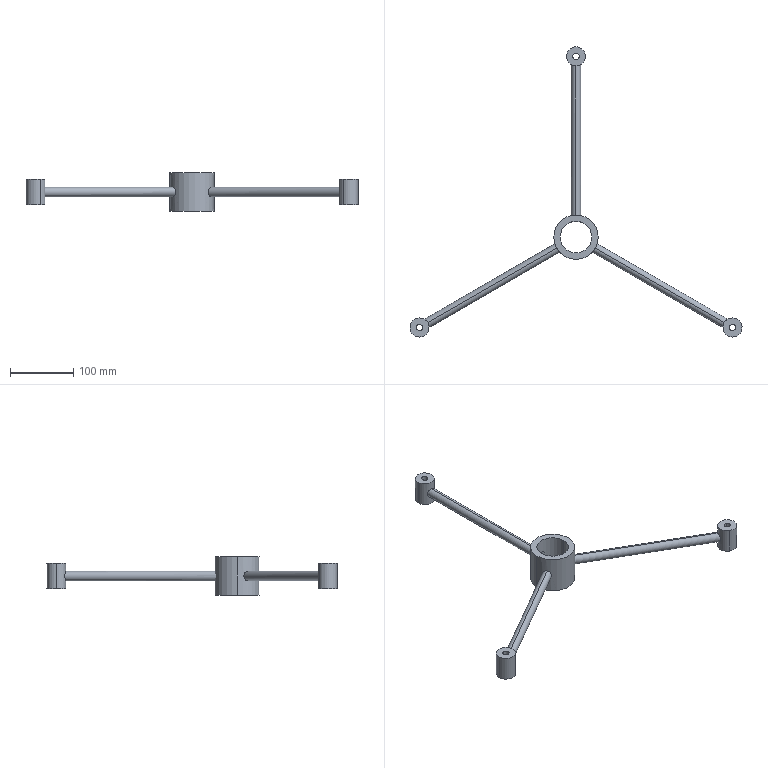Part | SolidWorks | features ICE 2, CirPattern 1, Extrusion 1 | 2 solids | 31 faces | box 523.634 x 457.5 x 60 mm | volume 315175 mm3 | cylinder 22 | plane 9 | commonest cylinder face diameters 10 x6 15 x6 30 x6 50 x2 70 x2
STEP:
#1=CARTESIAN_POINT('',(-5.,285.,20.));
#2=VERTEX_POINT('',#1);
#3=CARTESIAN_POINT('',(5.,285.,20.));
#4=VERTEX_POINT('',#3);
#5=CARTESIAN_POINT('',(0.,285.,20.));
#6=DIRECTION('',(0.,0.,1.));
#7=DIRECTION('',(1.,0.,0.));
#8=AXIS2_PLACEMENT_3D('',#5,#6,#7);
#9=CIRCLE('',#8,5.);
#10=EDGE_CURVE('',#2,#4,#9,.T.);
#11=ORIENTED_EDGE('',*,*,#10,.T.);
#12=CARTESIAN_POINT('',(5.,285.,-20.));
#13=VERTEX_POINT('',#12);
#14=CARTESIAN_POINT('',(5.,285.,20.));
#15=DIRECTION('',(0.,0.,-1.));
#16=VECTOR('',#15,1000.);
#17=LINE('',#14,#16);
#18=EDGE_CURVE('',#4,#13,#17,.T.);
#19=ORIENTED_EDGE('',*,*,#18,.T.);
#20=CARTESIAN_POINT('',(-5.,285.,-20.));
#21=VERTEX_POINT('',#20);
#22=CARTESIAN_POINT('',(0.,285.,-20.));
#23=DIRECTION('',(0.,0.,1.));
#24=DIRECTION('',(1.,0.,0.));
#25=AXIS2_PLACEMENT_3D('',#22,#23,#24);
#26=CIRCLE('',#25,5.);
#27=EDGE_CURVE('',#21,#13,#26,.T.);
#28=ORIENTED_EDGE('',*,*,#27,.F.);
#29=CARTESIAN_POINT('',(-5.,285.,20.));
#30=DIRECTION('',(0.,0.,-1.));
#31=VECTOR('',#30,1000.);
#32=LINE('',#29,#31);
#33=EDGE_CURVE('',#2,#21,#32,.T.);
#34=ORIENTED_EDGE('',*,*,#33,.F.);
#35=EDGE_LOOP('',(#11,#19,#28,#34));
#36=FACE_OUTER_BOUND('',#35,.T.);
#37=CARTESIAN_POINT('',(0.,285.,20.));
#38=DIRECTION('',(0.,0.,-1.));
#39=DIRECTION('',(-1.,0.,0.));
#40=AXIS2_PLACEMENT_3D('',#37,#38,#39);
#41=CYLINDRICAL_SURFACE('',#40,5.);
#42=ADVANCED_FACE('',(#36),#41,.F.);
#43=CARTESIAN_POINT('',(15.,285.,20.));
#44=VERTEX_POINT('',#43);
#45=CARTESIAN_POINT('',(-15.,285.,20.));
#46=VERTEX_POINT('',#45);
#47=CARTESIAN_POINT('',(0.,285.,20.));
#48=DIRECTION('',(0.,0.,1.));
#49=DIRECTION('',(1.,0.,0.));
#50=AXIS2_PLACEMENT_3D('',#47,#48,#49);
#51=CIRCLE('',#50,15.);
#52=EDGE_CURVE('',#44,#46,#51,.T.);
#53=ORIENTED_EDGE('',*,*,#52,.F.);
#54=CARTESIAN_POINT('',(15.,285.,-20.));
#55=VERTEX_POINT('',#54);
#56=CARTESIAN_POINT('',(15.,285.,20.));
#57=DIRECTION('',(0.,0.,-1.));
#58=VECTOR('',#57,1000.);
#59=LINE('',#56,#58);
#60=EDGE_CURVE('',#44,#55,#59,.T.);
#61=ORIENTED_EDGE('',*,*,#60,.T.);
#62=CARTESIAN_POINT('',(-15.,285.,-20.));
#63=VERTEX_POINT('',#62);
#64=CARTESIAN_POINT('',(0.,285.,-20.));
#65=DIRECTION('',(0.,0.,1.));
#66=DIRECTION('',(1.,0.,0.));
#67=AXIS2_PLACEMENT_3D('',#64,#65,#66);
#68=CIRCLE('',#67,15.);
#69=EDGE_CURVE('',#55,#63,#68,.T.);
#70=ORIENTED_EDGE('',*,*,#69,.T.);
#71=CARTESIAN_POINT('',(-15.,285.,20.));
#72=DIRECTION('',(0.,0.,-1.));
#73=VECTOR('',#72,1000.);
#74=LINE('',#71,#73);
#75=EDGE_CURVE('',#46,#63,#74,.T.);
#76=ORIENTED_EDGE('',*,*,#75,.F.);
#77=EDGE_LOOP('',(#53,#61,#70,#76));
#78=FACE_OUTER_BOUND('',#77,.T.);
#79=CARTESIAN_POINT('',(0.,285.,20.));
#80=DIRECTION('',(0.,0.,-1.));
#81=DIRECTION('',(-1.,0.,0.));
#82=AXIS2_PLACEMENT_3D('',#79,#80,#81);
#83=CYLINDRICAL_SURFACE('',#82,15.);
#84=ADVANCED_FACE('',(#78),#83,.T.);
#85=CARTESIAN_POINT('',(0.,270.,7.5));
#86=VERTEX_POINT('',#85);
#87=CARTESIAN_POINT('',(0.,270.,-7.5));
#88=VERTEX_POINT('',#87);
#89=CARTESIAN_POINT('',(0.,270.,7.5));
#90=CARTESIAN_POINT('',(0.4971,270.,7.5));
#91=CARTESIAN_POINT('',(1.003,270.026,7.449));
#92=CARTESIAN_POINT('',(1.975,270.123,7.252));
#93=CARTESIAN_POINT('',(2.446,270.193,7.107));
#94=CARTESIAN_POINT('',(3.36,270.374,6.724));
#95=CARTESIAN_POINT('',(3.789,270.48,6.491));
#96=CARTESIAN_POINT('',(4.592,270.714,5.949));
#97=CARTESIAN_POINT('',(4.97,270.843,5.637));
#98=CARTESIAN_POINT('',(5.651,271.1,4.955));
#99=CARTESIAN_POINT('',(5.956,271.23,4.584));
#100=CARTESIAN_POINT('',(6.361,271.415,3.981));
#101=CARTESIAN_POINT('',(6.488,271.475,3.771));
#102=CARTESIAN_POINT('',(6.719,271.588,3.341));
#103=CARTESIAN_POINT('',(6.824,271.642,3.122));
#104=CARTESIAN_POINT('',(7.105,271.788,2.449));
#105=CARTESIAN_POINT('',(7.251,271.868,1.982));
#106=CARTESIAN_POINT('',(7.4,271.952,1.248));
#107=CARTESIAN_POINT('',(7.437,271.974,0.999));
#108=CARTESIAN_POINT('',(7.487,272.002,0.5039));
#109=CARTESIAN_POINT('',(7.512,272.017,0.008359));
#110=CARTESIAN_POINT('',(7.488,272.003,-0.4882));
#111=CARTESIAN_POINT('',(7.439,271.975,-0.9852));
#112=CARTESIAN_POINT('',(7.402,271.953,-1.235));
#113=CARTESIAN_POINT('',(7.255,271.87,-1.967));
#114=CARTESIAN_POINT('',(7.11,271.79,-2.437));
#115=CARTESIAN_POINT('',(6.826,271.643,-3.117));
#116=CARTESIAN_POINT('',(6.719,271.589,-3.341));
#117=CARTESIAN_POINT('',(6.488,271.475,-3.77));
#118=CARTESIAN_POINT('',(6.363,271.416,-3.977));
#119=CARTESIAN_POINT('',(6.094,271.293,-4.379));
#120=CARTESIAN_POINT('',(5.95,271.23,-4.572));
#121=CARTESIAN_POINT('',(5.643,271.101,-4.946));
#122=CARTESIAN_POINT('',(5.479,271.035,-5.127));
#123=CARTESIAN_POINT('',(4.966,270.841,-5.641));
#124=CARTESIAN_POINT('',(4.595,270.715,-5.947));
#125=CARTESIAN_POINT('',(3.793,270.481,-6.488));
#126=CARTESIAN_POINT('',(3.356,270.373,-6.725));
#127=CARTESIAN_POINT('',(2.453,270.195,-7.105));
#128=CARTESIAN_POINT('',(1.984,270.124,-7.25));
#129=CARTESIAN_POINT('',(1.01,270.026,-7.448));
#130=CARTESIAN_POINT('',(0.5039,270.,-7.5));
#131=CARTESIAN_POINT('',(0.,270.,-7.5));
#132=B_SPLINE_CURVE_WITH_KNOTS('',3,(#89,#90,#91,#92,#93,#94,#95,#96,#97,#98,#99,#100,#101,#102,#103,#104,#105,#106,#107,#108,#109,#110,#111,#112,#113,#114,#115,#116,#117,#118,#119,#120,#121,#122,#123,#124,#125,#126,#127,#128,#129,#130,#131),.UNSPECIFIED.,.F.,.F.,(4,2,2,2,2,2,2,2,2,2,1,2,2,2,2,2,2,2,2,2,2,4),(0.02386,0.02535,0.02683,0.02832,0.02981,0.0313,0.03204,0.03279,0.03428,0.03502,0.03577,0.03651,0.03725,0.03874,0.03949,0.04023,0.04097,0.04172,0.04321,0.0447,0.04618,0.04767),.UNSPECIFIED.);
#133=EDGE_CURVE('',#86,#88,#132,.T.);
#134=ORIENTED_EDGE('',*,*,#133,.F.);
#135=CARTESIAN_POINT('',(0.,25.,7.5));
#136=VERTEX_POINT('',#135);
#137=CARTESIAN_POINT('',(0.,276.,7.5));
#138=DIRECTION('',(0.,-1.,0.));
#139=VECTOR('',#138,1000.);
#140=LINE('',#137,#139);
#141=EDGE_CURVE('',#86,#136,#140,.T.);
#142=ORIENTED_EDGE('',*,*,#141,.T.);
#143=CARTESIAN_POINT('',(0.,25.,-7.5));
#144=VERTEX_POINT('',#143);
#145=CARTESIAN_POINT('',(0.,25.,0.));
#146=DIRECTION('',(0.,1.,0.));
#147=DIRECTION('',(0.,0.,1.));
#148=AXIS2_PLACEMENT_3D('',#145,#146,#147);
#149=CIRCLE('',#148,7.5);
#150=EDGE_CURVE('',#136,#144,#149,.T.);
#151=ORIENTED_EDGE('',*,*,#150,.T.);
#152=CARTESIAN_POINT('',(0.,276.,-7.5));
#153=DIRECTION('',(0.,-1.,0.));
#154=VECTOR('',#153,1000.);
#155=LINE('',#152,#154);
#156=EDGE_CURVE('',#88,#144,#155,.T.);
#157=ORIENTED_EDGE('',*,*,#156,.F.);
#158=EDGE_LOOP('',(#134,#142,#151,#157));
#159=FACE_OUTER_BOUND('',#158,.T.);
#160=CARTESIAN_POINT('',(0.,276.,0.));
#161=DIRECTION('',(0.,-1.,0.));
#162=DIRECTION('',(0.,0.,-1.));
#163=AXIS2_PLACEMENT_3D('',#160,#161,#162);
#164=CYLINDRICAL_SURFACE('',#163,7.5);
#165=ADVANCED_FACE('',(#159),#164,.T.);
#166=ORIENTED_EDGE('',*,*,#141,.F.);
#167=CARTESIAN_POINT('',(0.,270.,-7.5));
#168=CARTESIAN_POINT('',(-0.5047,270.,-7.5));
#169=CARTESIAN_POINT('',(-0.9995,270.025,-7.45));
#170=CARTESIAN_POINT('',(-1.97,270.122,-7.253));
#171=CARTESIAN_POINT('',(-2.451,270.194,-7.105));
#172=CARTESIAN_POINT('',(-3.357,270.373,-6.725));
#173=CARTESIAN_POINT('',(-3.785,270.479,-6.493));
#174=CARTESIAN_POINT('',(-4.392,270.656,-6.084));
#175=CARTESIAN_POINT('',(-4.588,270.718,-5.938));
#176=CARTESIAN_POINT('',(-4.961,270.843,-5.63));
#177=CARTESIAN_POINT('',(-5.139,270.907,-5.468));
#178=CARTESIAN_POINT('',(-5.479,271.035,-5.127));
#179=CARTESIAN_POINT('',(-5.641,271.1,-4.949));
#180=CARTESIAN_POINT('',(-5.948,271.229,-4.575));
#181=CARTESIAN_POINT('',(-6.094,271.293,-4.379));
#182=CARTESIAN_POINT('',(-6.499,271.478,-3.774));
#183=CARTESIAN_POINT('',(-6.729,271.592,-3.348));
#184=CARTESIAN_POINT('',(-7.011,271.739,-2.675));
#185=CARTESIAN_POINT('',(-7.095,271.784,-2.444));
#186=CARTESIAN_POINT('',(-7.241,271.863,-1.97));
#187=CARTESIAN_POINT('',(-7.303,271.898,-1.727));
#188=CARTESIAN_POINT('',(-7.45,271.98,-0.9987));
#189=CARTESIAN_POINT('',(-7.5,272.009,-0.5064));
#190=CARTESIAN_POINT('',(-7.5,272.01,0.2423));
#191=CARTESIAN_POINT('',(-7.488,272.003,0.4954));
#192=CARTESIAN_POINT('',(-7.438,271.974,0.9943));
#193=CARTESIAN_POINT('',(-7.401,271.953,1.24));
#194=CARTESIAN_POINT('',(-7.303,271.898,1.726));
#195=CARTESIAN_POINT('',(-7.242,271.864,1.965));
#196=CARTESIAN_POINT('',(-7.097,271.785,2.437));
#197=CARTESIAN_POINT('',(-7.012,271.74,2.671));
#198=CARTESIAN_POINT('',(-6.727,271.591,3.352));
#199=CARTESIAN_POINT('',(-6.496,271.476,3.779));
#200=CARTESIAN_POINT('',(-6.09,271.291,4.384));
#201=CARTESIAN_POINT('',(-5.944,271.227,4.58));
#202=CARTESIAN_POINT('',(-5.636,271.098,4.954));
#203=CARTESIAN_POINT('',(-5.474,271.033,5.133));
#204=CARTESIAN_POINT('',(-4.964,270.84,5.643));
#205=CARTESIAN_POINT('',(-4.592,270.714,5.95));
#206=CARTESIAN_POINT('',(-3.779,270.478,6.497));
#207=CARTESIAN_POINT('',(-3.349,270.371,6.728));
#208=CARTESIAN_POINT('',(-2.674,270.238,7.011));
#209=CARTESIAN_POINT('',(-2.443,270.198,7.095));
#210=CARTESIAN_POINT('',(-1.971,270.128,7.241));
#211=CARTESIAN_POINT('',(-1.727,270.098,7.303));
#212=CARTESIAN_POINT('',(-0.9921,270.025,7.451));
#213=CARTESIAN_POINT('',(-0.498,270.,7.5));
#214=CARTESIAN_POINT('',(0.,270.,7.5));
#215=B_SPLINE_CURVE_WITH_KNOTS('',3,(#167,#168,#169,#170,#171,#172,#173,#174,#175,#176,#177,#178,#179,#180,#181,#182,#183,#184,#185,#186,#187,#188,#189,#190,#191,#192,#193,#194,#195,#196,#197,#198,#199,#200,#201,#202,#203,#204,#205,#206,#207,#208,#209,#210,#211,#212,#213,#214),.UNSPECIFIED.,.F.,.F.,(4,2,2,2,2,2,2,2,2,2,2,2,2,2,2,2,2,2,2,2,2,2,2,4),(0.,0.001491,0.002982,0.004473,0.005219,0.005964,0.00671,0.007455,0.008947,0.009692,0.01044,0.01193,0.01267,0.01342,0.01417,0.01491,0.0164,0.01715,0.01789,0.01938,0.02088,0.02162,0.02237,0.02386),.UNSPECIFIED.);
#216=EDGE_CURVE('',#88,#86,#215,.T.);
#217=ORIENTED_EDGE('',*,*,#216,.F.);
#218=ORIENTED_EDGE('',*,*,#156,.T.);
#219=CARTESIAN_POINT('',(0.,25.,0.));
#220=DIRECTION('',(0.,1.,0.));
#221=DIRECTION('',(0.,0.,1.));
#222=AXIS2_PLACEMENT_3D('',#219,#220,#221);
#223=CIRCLE('',#222,7.5);
#224=EDGE_CURVE('',#144,#136,#223,.T.);
#225=ORIENTED_EDGE('',*,*,#224,.T.);
#226=EDGE_LOOP('',(#166,#217,#218,#225));
#227=FACE_OUTER_BOUND('',#226,.T.);
#228=CARTESIAN_POINT('',(0.,276.,0.));
#229=DIRECTION('',(0.,-1.,0.));
#230=DIRECTION('',(0.,0.,-1.));
#231=AXIS2_PLACEMENT_3D('',#228,#229,#230);
#232=CYLINDRICAL_SURFACE('',#231,7.5);
#233=ADVANCED_FACE('',(#227),#232,.T.);
#234=ORIENTED_EDGE('',*,*,#224,.F.);
#235=ORIENTED_EDGE('',*,*,#150,.F.);
#236=EDGE_LOOP('',(#234,#235));
#237=FACE_OUTER_BOUND('',#236,.T.);
#238=CARTESIAN_POINT('',(0.,25.,0.));
#239=DIRECTION('',(0.,1.,0.));
#240=DIRECTION('',(0.,0.,1.));
#241=AXIS2_PLACEMENT_3D('',#238,#239,#240);
#242=PLANE('',#241);
#243=ADVANCED_FACE('',(#237),#242,.F.);
#244=ORIENTED_EDGE('',*,*,#60,.F.);
#245=CARTESIAN_POINT('',(0.,285.,20.));
#246=DIRECTION('',(0.,0.,1.));
#247=DIRECTION('',(1.,0.,0.));
#248=AXIS2_PLACEMENT_3D('',#245,#246,#247);
#249=CIRCLE('',#248,15.);
#250=EDGE_CURVE('',#46,#44,#249,.T.);
#251=ORIENTED_EDGE('',*,*,#250,.F.);
#252=ORIENTED_EDGE('',*,*,#75,.T.);
#253=CARTESIAN_POINT('',(0.,285.,-20.));
#254=DIRECTION('',(0.,0.,1.));
#255=DIRECTION('',(1.,0.,0.));
#256=AXIS2_PLACEMENT_3D('',#253,#254,#255);
#257=CIRCLE('',#256,15.);
#258=EDGE_CURVE('',#63,#55,#257,.T.);
#259=ORIENTED_EDGE('',*,*,#258,.T.);
#260=EDGE_LOOP('',(#244,#251,#252,#259));
#261=FACE_OUTER_BOUND('',#260,.T.);
#262=ORIENTED_EDGE('',*,*,#216,.T.);
#263=ORIENTED_EDGE('',*,*,#133,.T.);
#264=EDGE_LOOP('',(#262,#263));
#265=FACE_BOUND('',#264,.T.);
#266=CARTESIAN_POINT('',(0.,285.,20.));
#267=DIRECTION('',(0.,0.,-1.));
#268=DIRECTION('',(-1.,0.,0.));
#269=AXIS2_PLACEMENT_3D('',#266,#267,#268);
#270=CYLINDRICAL_SURFACE('',#269,15.);
#271=ADVANCED_FACE('',(#261,#265),#270,.T.);
#272=ORIENTED_EDGE('',*,*,#250,.T.);
#273=ORIENTED_EDGE('',*,*,#52,.T.);
#274=EDGE_LOOP('',(#272,#273));
#275=FACE_OUTER_BOUND('',#274,.T.);
#276=ORIENTED_EDGE('',*,*,#10,.F.);
#277=CARTESIAN_POINT('',(0.,285.,20.));
#278=DIRECTION('',(0.,0.,1.));
#279=DIRECTION('',(1.,0.,0.));
#280=AXIS2_PLACEMENT_3D('',#277,#278,#279);
#281=CIRCLE('',#280,5.);
#282=EDGE_CURVE('',#4,#2,#281,.T.);
#283=ORIENTED_EDGE('',*,*,#282,.F.);
#284=EDGE_LOOP('',(#276,#283));
#285=FACE_BOUND('',#284,.T.);
#286=CARTESIAN_POINT('',(0.,285.,20.));
#287=DIRECTION('',(0.,0.,1.));
#288=DIRECTION('',(1.,0.,0.));
#289=AXIS2_PLACEMENT_3D('',#286,#287,#288);
#290=PLANE('',#289);
#291=ADVANCED_FACE('',(#275,#285),#290,.T.);
#292=ORIENTED_EDGE('',*,*,#258,.F.);
#293=ORIENTED_EDGE('',*,*,#69,.F.);
#294=EDGE_LOOP('',(#292,#293));
#295=FACE_OUTER_BOUND('',#294,.T.);
#296=ORIENTED_EDGE('',*,*,#27,.T.);
#297=CARTESIAN_POINT('',(0.,285.,-20.));
#298=DIRECTION('',(0.,0.,1.));
#299=DIRECTION('',(1.,0.,0.));
#300=AXIS2_PLACEMENT_3D('',#297,#298,#299);
#301=CIRCLE('',#300,5.);
#302=EDGE_CURVE('',#13,#21,#301,.T.);
#303=ORIENTED_EDGE('',*,*,#302,.T.);
#304=EDGE_LOOP('',(#296,#303));
#305=FACE_BOUND('',#304,.T.);
#306=CARTESIAN_POINT('',(0.,285.,-20.));
#307=DIRECTION('',(0.,0.,1.));
#308=DIRECTION('',(1.,0.,0.));
#309=AXIS2_PLACEMENT_3D('',#306,#307,#308);
#310=PLANE('',#309);
#311=ADVANCED_FACE('',(#295,#305),#310,.F.);
#312=ORIENTED_EDGE('',*,*,#18,.F.);
#313=ORIENTED_EDGE('',*,*,#282,.T.);
#314=ORIENTED_EDGE('',*,*,#33,.T.);
#315=ORIENTED_EDGE('',*,*,#302,.F.);
#316=EDGE_LOOP('',(#312,#313,#314,#315));
#317=FACE_OUTER_BOUND('',#316,.T.);
#318=CARTESIAN_POINT('',(0.,285.,20.));
#319=DIRECTION('',(0.,0.,-1.));
#320=DIRECTION('',(-1.,0.,0.));
#321=AXIS2_PLACEMENT_3D('',#318,#319,#320);
#322=CYLINDRICAL_SURFACE('',#321,5.);
#323=ADVANCED_FACE('',(#317),#322,.F.);
#324=CLOSED_SHELL('',(#42,#84,#165,#233,#243,#271,#291,#311,#323));
#325=MANIFOLD_SOLID_BREP('',#324);
#326=CARTESIAN_POINT('',(-244.317,-146.83,20.));
#327=VERTEX_POINT('',#326);
#328=CARTESIAN_POINT('',(-249.317,-138.17,20.));
#329=VERTEX_POINT('',#328);
#330=CARTESIAN_POINT('',(-246.817,-142.5,20.));
#331=DIRECTION('',(0.,0.,1.));
#332=DIRECTION('',(-0.5,0.866,0.));
#333=AXIS2_PLACEMENT_3D('',#330,#331,#332);
#334=CIRCLE('',#333,5.);
#335=EDGE_CURVE('',#327,#329,#334,.T.);
#336=ORIENTED_EDGE('',*,*,#335,.T.);
#337=CARTESIAN_POINT('',(-249.317,-138.17,-20.));
#338=VERTEX_POINT('',#337);
#339=CARTESIAN_POINT('',(-249.317,-138.17,20.));
#340=DIRECTION('',(0.,0.,-1.));
#341=VECTOR('',#340,1000.);
#342=LINE('',#339,#341);
#343=EDGE_CURVE('',#329,#338,#342,.T.);
#344=ORIENTED_EDGE('',*,*,#343,.T.);
#345=CARTESIAN_POINT('',(-244.317,-146.83,-20.));
#346=VERTEX_POINT('',#345);
#347=CARTESIAN_POINT('',(-246.817,-142.5,-20.));
#348=DIRECTION('',(0.,0.,1.));
#349=DIRECTION('',(-0.5,0.866,0.));
#350=AXIS2_PLACEMENT_3D('',#347,#348,#349);
#351=CIRCLE('',#350,5.);
#352=EDGE_CURVE('',#346,#338,#351,.T.);
#353=ORIENTED_EDGE('',*,*,#352,.F.);
#354=CARTESIAN_POINT('',(-244.317,-146.83,20.));
#355=DIRECTION('',(0.,0.,-1.));
#356=VECTOR('',#355,1000.);
#357=LINE('',#354,#356);
#358=EDGE_CURVE('',#327,#346,#357,.T.);
#359=ORIENTED_EDGE('',*,*,#358,.F.);
#360=EDGE_LOOP('',(#336,#344,#353,#359));
#361=FACE_OUTER_BOUND('',#360,.T.);
#362=CARTESIAN_POINT('',(-246.817,-142.5,20.));
#363=DIRECTION('',(0.,0.,-1.));
#364=DIRECTION('',(0.5,-0.866,0.));
#365=AXIS2_PLACEMENT_3D('',#362,#363,#364);
#366=CYLINDRICAL_SURFACE('',#365,5.);
#367=ADVANCED_FACE('',(#361),#366,.F.);
#368=CARTESIAN_POINT('',(-254.317,-129.51,20.));
#369=VERTEX_POINT('',#368);
#370=CARTESIAN_POINT('',(-239.317,-155.49,20.));
#371=VERTEX_POINT('',#370);
#372=CARTESIAN_POINT('',(-246.817,-142.5,20.));
#373=DIRECTION('',(0.,0.,1.));
#374=DIRECTION('',(-0.5,0.866,0.));
#375=AXIS2_PLACEMENT_3D('',#372,#373,#374);
#376=CIRCLE('',#375,15.);
#377=EDGE_CURVE('',#369,#371,#376,.T.);
#378=ORIENTED_EDGE('',*,*,#377,.F.);
#379=CARTESIAN_POINT('',(-254.317,-129.51,-20.));
#380=VERTEX_POINT('',#379);
#381=CARTESIAN_POINT('',(-254.317,-129.51,20.));
#382=DIRECTION('',(0.,0.,-1.));
#383=VECTOR('',#382,1000.);
#384=LINE('',#381,#383);
#385=EDGE_CURVE('',#369,#380,#384,.T.);
#386=ORIENTED_EDGE('',*,*,#385,.T.);
#387=CARTESIAN_POINT('',(-239.317,-155.49,-20.));
#388=VERTEX_POINT('',#387);
#389=CARTESIAN_POINT('',(-246.817,-142.5,-20.));
#390=DIRECTION('',(0.,0.,1.));
#391=DIRECTION('',(-0.5,0.866,0.));
#392=AXIS2_PLACEMENT_3D('',#389,#390,#391);
#393=CIRCLE('',#392,15.);
#394=EDGE_CURVE('',#380,#388,#393,.T.);
#395=ORIENTED_EDGE('',*,*,#394,.T.);
#396=CARTESIAN_POINT('',(-239.317,-155.49,20.));
#397=DIRECTION('',(0.,0.,-1.));
#398=VECTOR('',#397,1000.);
#399=LINE('',#396,#398);
#400=EDGE_CURVE('',#371,#388,#399,.T.);
#401=ORIENTED_EDGE('',*,*,#400,.F.);
#402=EDGE_LOOP('',(#378,#386,#395,#401));
#403=FACE_OUTER_BOUND('',#402,.T.);
#404=CARTESIAN_POINT('',(-246.817,-142.5,20.));
#405=DIRECTION('',(0.,0.,-1.));
#406=DIRECTION('',(0.5,-0.866,0.));
#407=AXIS2_PLACEMENT_3D('',#404,#405,#406);
#408=CYLINDRICAL_SURFACE('',#407,15.);
#409=ADVANCED_FACE('',(#403),#408,.T.);
#410=CARTESIAN_POINT('',(-233.827,-135.,7.5));
#411=VERTEX_POINT('',#410);
#412=CARTESIAN_POINT('',(-233.827,-135.,-7.5));
#413=VERTEX_POINT('',#412);
#414=CARTESIAN_POINT('',(-233.827,-135.,7.5));
#415=CARTESIAN_POINT('',(-234.075,-134.569,7.5));
#416=CARTESIAN_POINT('',(-234.351,-134.144,7.449));
#417=CARTESIAN_POINT('',(-234.921,-133.351,7.252));
#418=CARTESIAN_POINT('',(-235.218,-132.978,7.107));
#419=CARTESIAN_POINT('',(-235.83,-132.277,6.724));
#420=CARTESIAN_POINT('',(-236.137,-131.959,6.491));
#421=CARTESIAN_POINT('',(-236.741,-131.38,5.949));
#422=CARTESIAN_POINT('',(-237.042,-131.117,5.637));
#423=CARTESIAN_POINT('',(-237.605,-130.656,4.955));
#424=CARTESIAN_POINT('',(-237.87,-130.457,4.584));
#425=CARTESIAN_POINT('',(-238.233,-130.199,3.981));
#426=CARTESIAN_POINT('',(-238.348,-130.119,3.771));
#427=CARTESIAN_POINT('',(-238.562,-129.975,3.341));
#428=CARTESIAN_POINT('',(-238.66,-129.911,3.122));
#429=CARTESIAN_POINT('',(-238.928,-129.74,2.449));
#430=CARTESIAN_POINT('',(-239.07,-129.655,1.982));
#431=CARTESIAN_POINT('',(-239.217,-129.568,1.248));
#432=CARTESIAN_POINT('',(-239.255,-129.546,0.999));
#433=CARTESIAN_POINT('',(-239.304,-129.517,0.5039));
#434=CARTESIAN_POINT('',(-239.33,-129.503,0.008359));
#435=CARTESIAN_POINT('',(-239.305,-129.516,-0.4882));
#436=CARTESIAN_POINT('',(-239.257,-129.545,-0.9852));
#437=CARTESIAN_POINT('',(-239.219,-129.567,-1.235));
#438=CARTESIAN_POINT('',(-239.074,-129.653,-1.967));
#439=CARTESIAN_POINT('',(-238.932,-129.738,-2.437));
#440=CARTESIAN_POINT('',(-238.662,-129.91,-3.117));
#441=CARTESIAN_POINT('',(-238.562,-129.975,-3.341));
#442=CARTESIAN_POINT('',(-238.349,-130.119,-3.77));
#443=CARTESIAN_POINT('',(-238.234,-130.197,-3.977));
#444=CARTESIAN_POINT('',(-237.994,-130.369,-4.379));
#445=CARTESIAN_POINT('',(-237.867,-130.462,-4.572));
#446=CARTESIAN_POINT('',(-237.602,-130.663,-4.946));
#447=CARTESIAN_POINT('',(-237.463,-130.773,-5.127));
#448=CARTESIAN_POINT('',(-237.039,-131.12,-5.641));
#449=CARTESIAN_POINT('',(-236.744,-131.378,-5.947));
#450=CARTESIAN_POINT('',(-236.14,-131.956,-6.488));
#451=CARTESIAN_POINT('',(-235.828,-132.28,-6.725));
#452=CARTESIAN_POINT('',(-235.222,-132.973,-7.105));
#453=CARTESIAN_POINT('',(-234.926,-133.344,-7.25));
#454=CARTESIAN_POINT('',(-234.355,-134.138,-7.448));
#455=CARTESIAN_POINT('',(-234.079,-134.564,-7.5));
#456=CARTESIAN_POINT('',(-233.827,-135.,-7.5));
#457=B_SPLINE_CURVE_WITH_KNOTS('',3,(#414,#415,#416,#417,#418,#419,#420,#421,#422,#423,#424,#425,#426,#427,#428,#429,#430,#431,#432,#433,#434,#435,#436,#437,#438,#439,#440,#441,#442,#443,#444,#445,#446,#447,#448,#449,#450,#451,#452,#453,#454,#455,#456),.UNSPECIFIED.,.F.,.F.,(4,2,2,2,2,2,2,2,2,2,1,2,2,2,2,2,2,2,2,2,2,4),(0.02386,0.02535,0.02683,0.02832,0.02981,0.0313,0.03204,0.03279,0.03428,0.03502,0.03577,0.03651,0.03725,0.03874,0.03949,0.04023,0.04097,0.04172,0.04321,0.0447,0.04618,0.04767),.UNSPECIFIED.);
#458=EDGE_CURVE('',#411,#413,#457,.T.);
#459=ORIENTED_EDGE('',*,*,#458,.F.);
#460=CARTESIAN_POINT('',(-30.311,-17.5,7.5));
#461=VERTEX_POINT('',#460);
#462=CARTESIAN_POINT('',(-239.023,-138.,7.5));
#463=DIRECTION('',(0.866,0.5,0.));
#464=VECTOR('',#463,1000.);
#465=LINE('',#462,#464);
#466=EDGE_CURVE('',#411,#461,#465,.T.);
#467=ORIENTED_EDGE('',*,*,#466,.T.);
#468=CARTESIAN_POINT('',(-30.311,-17.5,-7.5));
#469=VERTEX_POINT('',#468);
#470=CARTESIAN_POINT('',(-30.311,-17.5,7.5));
#471=CARTESIAN_POINT('',(-30.556,-17.076,7.5));
#472=CARTESIAN_POINT('',(-30.791,-16.648,7.452));
#473=CARTESIAN_POINT('',(-31.242,-15.785,7.259));
#474=CARTESIAN_POINT('',(-31.451,-15.363,7.115));
#475=CARTESIAN_POINT('',(-31.742,-14.748,6.834));
#476=CARTESIAN_POINT('',(-31.835,-14.546,6.73));
#477=CARTESIAN_POINT('',(-32.013,-14.149,6.498));
#478=CARTESIAN_POINT('',(-32.099,-13.953,6.37));
#479=CARTESIAN_POINT('',(-32.342,-13.386,5.961));
#480=CARTESIAN_POINT('',(-32.485,-13.034,5.652));
#481=CARTESIAN_POINT('',(-32.739,-12.382,4.961));
#482=CARTESIAN_POINT('',(-32.85,-12.081,4.576));
#483=CARTESIAN_POINT('',(-33.036,-11.562,3.765));
#484=CARTESIAN_POINT('',(-33.113,-11.34,3.335));
#485=CARTESIAN_POINT('',(-33.205,-11.065,2.652));
#486=CARTESIAN_POINT('',(-33.232,-10.984,2.418));
#487=CARTESIAN_POINT('',(-33.278,-10.845,1.948));
#488=CARTESIAN_POINT('',(-33.315,-10.729,1.473));
#489=CARTESIAN_POINT('',(-33.338,-10.658,0.9887));
#490=CARTESIAN_POINT('',(-33.353,-10.611,0.4994));
#491=CARTESIAN_POINT('',(-33.357,-10.598,0.2509));
#492=CARTESIAN_POINT('',(-33.357,-10.598,-0.4916));
#493=CARTESIAN_POINT('',(-33.342,-10.645,-0.9795));
#494=CARTESIAN_POINT('',(-33.282,-10.831,-1.941));
#495=CARTESIAN_POINT('',(-33.236,-10.972,-2.42));
#496=CARTESIAN_POINT('',(-33.114,-11.335,-3.325));
#497=CARTESIAN_POINT('',(-33.038,-11.557,-3.756));
#498=CARTESIAN_POINT('',(-32.898,-11.948,-4.368));
#499=CARTESIAN_POINT('',(-32.846,-12.089,-4.568));
#500=CARTESIAN_POINT('',(-32.736,-12.385,-4.947));
#501=CARTESIAN_POINT('',(-32.677,-12.54,-5.128));
#502=CARTESIAN_POINT('',(-32.487,-13.027,-5.645));
#503=CARTESIAN_POINT('',(-32.344,-13.38,-5.956));
#504=CARTESIAN_POINT('',(-32.019,-14.14,-6.506));
#505=CARTESIAN_POINT('',(-31.842,-14.535,-6.736));
#506=CARTESIAN_POINT('',(-31.552,-15.149,-7.018));
#507=CARTESIAN_POINT('',(-31.452,-15.357,-7.101));
#508=CARTESIAN_POINT('',(-31.241,-15.781,-7.245));
#509=CARTESIAN_POINT('',(-31.132,-15.996,-7.306));
#510=CARTESIAN_POINT('',(-30.795,-16.64,-7.451));
#511=CARTESIAN_POINT('',(-30.559,-17.07,-7.5));
#512=CARTESIAN_POINT('',(-30.311,-17.5,-7.5));
#513=B_SPLINE_CURVE_WITH_KNOTS('',3,(#470,#471,#472,#473,#474,#475,#476,#477,#478,#479,#480,#481,#482,#483,#484,#485,#486,#487,#488,#489,#490,#491,#492,#493,#494,#495,#496,#497,#498,#499,#500,#501,#502,#503,#504,#505,#506,#507,#508,#509,#510,#511,#512),.UNSPECIFIED.,.F.,.F.,(4,2,2,2,2,2,2,2,2,1,2,2,2,2,2,2,2,2,2,2,2,4),(0.02352,0.02499,0.02646,0.02719,0.02792,0.02939,0.03086,0.03233,0.03307,0.0338,0.03454,0.03527,0.03674,0.03821,0.03968,0.04041,0.04115,0.04262,0.04409,0.04482,0.04556,0.04703),.UNSPECIFIED.);
#514=EDGE_CURVE('',#461,#469,#513,.T.);
#515=ORIENTED_EDGE('',*,*,#514,.T.);
#516=CARTESIAN_POINT('',(-239.023,-138.,-7.5));
#517=DIRECTION('',(0.866,0.5,0.));
#518=VECTOR('',#517,1000.);
#519=LINE('',#516,#518);
#520=EDGE_CURVE('',#413,#469,#519,.T.);
#521=ORIENTED_EDGE('',*,*,#520,.F.);
#522=EDGE_LOOP('',(#459,#467,#515,#521));
#523=FACE_OUTER_BOUND('',#522,.T.);
#524=CARTESIAN_POINT('',(-239.023,-138.,0.));
#525=DIRECTION('',(0.866,0.5,0.));
#526=DIRECTION('',(0.,0.,-1.));
#527=AXIS2_PLACEMENT_3D('',#524,#525,#526);
#528=CYLINDRICAL_SURFACE('',#527,7.5);
#529=ADVANCED_FACE('',(#523),#528,.T.);
#530=CARTESIAN_POINT('',(249.317,-138.17,20.));
#531=VERTEX_POINT('',#530);
#532=CARTESIAN_POINT('',(244.317,-146.83,20.));
#533=VERTEX_POINT('',#532);
#534=CARTESIAN_POINT('',(246.817,-142.5,20.));
#535=DIRECTION('',(0.,0.,1.));
#536=DIRECTION('',(-0.5,-0.866,0.));
#537=AXIS2_PLACEMENT_3D('',#534,#535,#536);
#538=CIRCLE('',#537,5.);
#539=EDGE_CURVE('',#531,#533,#538,.T.);
#540=ORIENTED_EDGE('',*,*,#539,.T.);
#541=CARTESIAN_POINT('',(244.317,-146.83,-20.));
#542=VERTEX_POINT('',#541);
#543=CARTESIAN_POINT('',(244.317,-146.83,20.));
#544=DIRECTION('',(0.,0.,-1.));
#545=VECTOR('',#544,1000.);
#546=LINE('',#543,#545);
#547=EDGE_CURVE('',#533,#542,#546,.T.);
#548=ORIENTED_EDGE('',*,*,#547,.T.);
#549=CARTESIAN_POINT('',(249.317,-138.17,-20.));
#550=VERTEX_POINT('',#549);
#551=CARTESIAN_POINT('',(246.817,-142.5,-20.));
#552=DIRECTION('',(0.,0.,1.));
#553=DIRECTION('',(-0.5,-0.866,0.));
#554=AXIS2_PLACEMENT_3D('',#551,#552,#553);
#555=CIRCLE('',#554,5.);
#556=EDGE_CURVE('',#550,#542,#555,.T.);
#557=ORIENTED_EDGE('',*,*,#556,.F.);
#558=CARTESIAN_POINT('',(249.317,-138.17,20.));
#559=DIRECTION('',(0.,0.,-1.));
#560=VECTOR('',#559,1000.);
#561=LINE('',#558,#560);
#562=EDGE_CURVE('',#531,#550,#561,.T.);
#563=ORIENTED_EDGE('',*,*,#562,.F.);
#564=EDGE_LOOP('',(#540,#548,#557,#563));
#565=FACE_OUTER_BOUND('',#564,.T.);
#566=CARTESIAN_POINT('',(246.817,-142.5,20.));
#567=DIRECTION('',(0.,0.,-1.));
#568=DIRECTION('',(0.5,0.866,0.));
#569=AXIS2_PLACEMENT_3D('',#566,#567,#568);
#570=CYLINDRICAL_SURFACE('',#569,5.);
#571=ADVANCED_FACE('',(#565),#570,.F.);
#572=CARTESIAN_POINT('',(239.317,-155.49,20.));
#573=VERTEX_POINT('',#572);
#574=CARTESIAN_POINT('',(254.317,-129.51,20.));
#575=VERTEX_POINT('',#574);
#576=CARTESIAN_POINT('',(246.817,-142.5,20.));
#577=DIRECTION('',(0.,0.,1.));
#578=DIRECTION('',(-0.5,-0.866,0.));
#579=AXIS2_PLACEMENT_3D('',#576,#577,#578);
#580=CIRCLE('',#579,15.);
#581=EDGE_CURVE('',#573,#575,#580,.T.);
#582=ORIENTED_EDGE('',*,*,#581,.F.);
#583=CARTESIAN_POINT('',(239.317,-155.49,-20.));
#584=VERTEX_POINT('',#583);
#585=CARTESIAN_POINT('',(239.317,-155.49,20.));
#586=DIRECTION('',(0.,0.,-1.));
#587=VECTOR('',#586,1000.);
#588=LINE('',#585,#587);
#589=EDGE_CURVE('',#573,#584,#588,.T.);
#590=ORIENTED_EDGE('',*,*,#589,.T.);
#591=CARTESIAN_POINT('',(254.317,-129.51,-20.));
#592=VERTEX_POINT('',#591);
#593=CARTESIAN_POINT('',(246.817,-142.5,-20.));
#594=DIRECTION('',(0.,0.,1.));
#595=DIRECTION('',(-0.5,-0.866,0.));
#596=AXIS2_PLACEMENT_3D('',#593,#594,#595);
#597=CIRCLE('',#596,15.);
#598=EDGE_CURVE('',#584,#592,#597,.T.);
#599=ORIENTED_EDGE('',*,*,#598,.T.);
#600=CARTESIAN_POINT('',(254.317,-129.51,20.));
#601=DIRECTION('',(0.,0.,-1.));
#602=VECTOR('',#601,1000.);
#603=LINE('',#600,#602);
#604=EDGE_CURVE('',#575,#592,#603,.T.);
#605=ORIENTED_EDGE('',*,*,#604,.F.);
#606=EDGE_LOOP('',(#582,#590,#599,#605));
#607=FACE_OUTER_BOUND('',#606,.T.);
#608=CARTESIAN_POINT('',(246.817,-142.5,20.));
#609=DIRECTION('',(0.,0.,-1.));
#610=DIRECTION('',(0.5,0.866,0.));
#611=AXIS2_PLACEMENT_3D('',#608,#609,#610);
#612=CYLINDRICAL_SURFACE('',#611,15.);
#613=ADVANCED_FACE('',(#607),#612,.T.);
#614=CARTESIAN_POINT('',(233.827,-135.,7.5));
#615=VERTEX_POINT('',#614);
#616=CARTESIAN_POINT('',(233.827,-135.,-7.5));
#617=VERTEX_POINT('',#616);
#618=CARTESIAN_POINT('',(233.827,-135.,7.5));
#619=CARTESIAN_POINT('',(233.578,-135.431,7.5));
#620=CARTESIAN_POINT('',(233.348,-135.881,7.449));
#621=CARTESIAN_POINT('',(232.945,-136.772,7.252));
#622=CARTESIAN_POINT('',(232.771,-137.215,7.107));
#623=CARTESIAN_POINT('',(232.471,-138.097,6.724));
#624=CARTESIAN_POINT('',(232.348,-138.521,6.491));
#625=CARTESIAN_POINT('',(232.149,-139.334,5.949));
#626=CARTESIAN_POINT('',(232.072,-139.726,5.637));
#627=CARTESIAN_POINT('',(231.954,-140.444,4.955));
#628=CARTESIAN_POINT('',(231.914,-140.773,4.584));
#629=CARTESIAN_POINT('',(231.872,-141.216,3.981));
#630=CARTESIAN_POINT('',(231.86,-141.356,3.771));
#631=CARTESIAN_POINT('',(231.843,-141.613,3.341));
#632=CARTESIAN_POINT('',(231.837,-141.73,3.122));
#633=CARTESIAN_POINT('',(231.823,-142.048,2.449));
#634=CARTESIAN_POINT('',(231.82,-142.213,1.982));
#635=CARTESIAN_POINT('',(231.818,-142.384,1.248));
#636=CARTESIAN_POINT('',(231.817,-142.428,0.999));
#637=CARTESIAN_POINT('',(231.817,-142.485,0.5039));
#638=CARTESIAN_POINT('',(231.817,-142.514,0.008359));
#639=CARTESIAN_POINT('',(231.817,-142.486,-0.4882));
#640=CARTESIAN_POINT('',(231.817,-142.43,-0.9852));
#641=CARTESIAN_POINT('',(231.818,-142.387,-1.235));
#642=CARTESIAN_POINT('',(231.819,-142.218,-1.967));
#643=CARTESIAN_POINT('',(231.822,-142.053,-2.437));
#644=CARTESIAN_POINT('',(231.837,-141.733,-3.117));
#645=CARTESIAN_POINT('',(231.843,-141.613,-3.341));
#646=CARTESIAN_POINT('',(231.86,-141.357,-3.77));
#647=CARTESIAN_POINT('',(231.871,-141.218,-3.977));
#648=CARTESIAN_POINT('',(231.9,-140.924,-4.379));
#649=CARTESIAN_POINT('',(231.917,-140.768,-4.572));
#650=CARTESIAN_POINT('',(231.959,-140.437,-4.946));
#651=CARTESIAN_POINT('',(231.984,-140.263,-5.127));
#652=CARTESIAN_POINT('',(232.072,-139.722,-5.641));
#653=CARTESIAN_POINT('',(232.149,-139.337,-5.947));
#654=CARTESIAN_POINT('',(232.347,-138.525,-6.488));
#655=CARTESIAN_POINT('',(232.472,-138.093,-6.725));
#656=CARTESIAN_POINT('',(232.769,-137.221,-7.105));
#657=CARTESIAN_POINT('',(232.942,-136.78,-7.25));
#658=CARTESIAN_POINT('',(233.344,-135.888,-7.448));
#659=CARTESIAN_POINT('',(233.575,-135.436,-7.5));
#660=CARTESIAN_POINT('',(233.827,-135.,-7.5));
#661=B_SPLINE_CURVE_WITH_KNOTS('',3,(#618,#619,#620,#621,#622,#623,#624,#625,#626,#627,#628,#629,#630,#631,#632,#633,#634,#635,#636,#637,#638,#639,#640,#641,#642,#643,#644,#645,#646,#647,#648,#649,#650,#651,#652,#653,#654,#655,#656,#657,#658,#659,#660),.UNSPECIFIED.,.F.,.F.,(4,2,2,2,2,2,2,2,2,2,1,2,2,2,2,2,2,2,2,2,2,4),(0.02386,0.02535,0.02683,0.02832,0.02981,0.0313,0.03204,0.03279,0.03428,0.03502,0.03577,0.03651,0.03725,0.03874,0.03949,0.04023,0.04097,0.04172,0.04321,0.0447,0.04618,0.04767),.UNSPECIFIED.);
#662=EDGE_CURVE('',#615,#617,#661,.T.);
#663=ORIENTED_EDGE('',*,*,#662,.F.);
#664=CARTESIAN_POINT('',(30.311,-17.5,7.5));
#665=VERTEX_POINT('',#664);
#666=CARTESIAN_POINT('',(239.023,-138.,7.5));
#667=DIRECTION('',(-0.866,0.5,0.));
#668=VECTOR('',#667,1000.);
#669=LINE('',#666,#668);
#670=EDGE_CURVE('',#615,#665,#669,.T.);
#671=ORIENTED_EDGE('',*,*,#670,.T.);
#672=CARTESIAN_POINT('',(30.311,-17.5,-7.5));
#673=VERTEX_POINT('',#672);
#674=CARTESIAN_POINT('',(30.311,-17.5,7.5));
#675=CARTESIAN_POINT('',(30.066,-17.924,7.5));
#676=CARTESIAN_POINT('',(29.813,-18.342,7.452));
#677=CARTESIAN_POINT('',(29.291,-19.164,7.259));
#678=CARTESIAN_POINT('',(29.03,-19.556,7.115));
#679=CARTESIAN_POINT('',(28.643,-20.115,6.834));
#680=CARTESIAN_POINT('',(28.515,-20.297,6.73));
#681=CARTESIAN_POINT('',(28.26,-20.65,6.498));
#682=CARTESIAN_POINT('',(28.133,-20.823,6.37));
#683=CARTESIAN_POINT('',(27.764,-21.316,5.961));
#684=CARTESIAN_POINT('',(27.53,-21.616,5.652));
#685=CARTESIAN_POINT('',(27.092,-22.162,4.961));
#686=CARTESIAN_POINT('',(26.888,-22.408,4.576));
#687=CARTESIAN_POINT('',(26.531,-22.829,3.765));
#688=CARTESIAN_POINT('',(26.377,-23.007,3.335));
#689=CARTESIAN_POINT('',(26.185,-23.224,2.652));
#690=CARTESIAN_POINT('',(26.128,-23.288,2.418));
#691=CARTESIAN_POINT('',(26.031,-23.397,1.948));
#692=CARTESIAN_POINT('',(25.949,-23.487,1.473));
#693=CARTESIAN_POINT('',(25.899,-23.542,0.9887));
#694=CARTESIAN_POINT('',(25.866,-23.579,0.4994));
#695=CARTESIAN_POINT('',(25.857,-23.589,0.2509));
#696=CARTESIAN_POINT('',(25.857,-23.589,-0.4916));
#697=CARTESIAN_POINT('',(25.89,-23.552,-0.9795));
#698=CARTESIAN_POINT('',(26.021,-23.408,-1.941));
#699=CARTESIAN_POINT('',(26.12,-23.297,-2.42));
#700=CARTESIAN_POINT('',(26.374,-23.01,-3.325));
#701=CARTESIAN_POINT('',(26.528,-22.833,-3.756));
#702=CARTESIAN_POINT('',(26.796,-22.516,-4.368));
#703=CARTESIAN_POINT('',(26.893,-22.401,-4.568));
#704=CARTESIAN_POINT('',(27.093,-22.158,-4.947));
#705=CARTESIAN_POINT('',(27.198,-22.029,-5.128));
#706=CARTESIAN_POINT('',(27.525,-21.622,-5.645));
#707=CARTESIAN_POINT('',(27.76,-21.321,-5.956));
#708=CARTESIAN_POINT('',(28.255,-20.659,-6.506));
#709=CARTESIAN_POINT('',(28.509,-20.309,-6.736));
#710=CARTESIAN_POINT('',(28.896,-19.751,-7.018));
#711=CARTESIAN_POINT('',(29.026,-19.559,-7.101));
#712=CARTESIAN_POINT('',(29.287,-19.166,-7.245));
#713=CARTESIAN_POINT('',(29.419,-18.963,-7.306));
#714=CARTESIAN_POINT('',(29.808,-18.35,-7.451));
#715=CARTESIAN_POINT('',(30.062,-17.93,-7.5));
#716=CARTESIAN_POINT('',(30.311,-17.5,-7.5));
#717=B_SPLINE_CURVE_WITH_KNOTS('',3,(#674,#675,#676,#677,#678,#679,#680,#681,#682,#683,#684,#685,#686,#687,#688,#689,#690,#691,#692,#693,#694,#695,#696,#697,#698,#699,#700,#701,#702,#703,#704,#705,#706,#707,#708,#709,#710,#711,#712,#713,#714,#715,#716),.UNSPECIFIED.,.F.,.F.,(4,2,2,2,2,2,2,2,2,1,2,2,2,2,2,2,2,2,2,2,2,4),(0.02352,0.02499,0.02646,0.02719,0.02792,0.02939,0.03086,0.03233,0.03307,0.0338,0.03454,0.03527,0.03674,0.03821,0.03968,0.04041,0.04115,0.04262,0.04409,0.04482,0.04556,0.04703),.UNSPECIFIED.);
#718=EDGE_CURVE('',#665,#673,#717,.T.);
#719=ORIENTED_EDGE('',*,*,#718,.T.);
#720=CARTESIAN_POINT('',(239.023,-138.,-7.5));
#721=DIRECTION('',(-0.866,0.5,0.));
#722=VECTOR('',#721,1000.);
#723=LINE('',#720,#722);
#724=EDGE_CURVE('',#617,#673,#723,.T.);
#725=ORIENTED_EDGE('',*,*,#724,.F.);
#726=EDGE_LOOP('',(#663,#671,#719,#725));
#727=FACE_OUTER_BOUND('',#726,.T.);
#728=CARTESIAN_POINT('',(239.023,-138.,0.));
#729=DIRECTION('',(-0.866,0.5,0.));
#730=DIRECTION('',(0.,0.,-1.));
#731=AXIS2_PLACEMENT_3D('',#728,#729,#730);
#732=CYLINDRICAL_SURFACE('',#731,7.5);
#733=ADVANCED_FACE('',(#727),#732,.T.);
#734=CARTESIAN_POINT('',(-25.,0.,30.));
#735=VERTEX_POINT('',#734);
#736=CARTESIAN_POINT('',(25.,0.,30.));
#737=VERTEX_POINT('',#736);
#738=CARTESIAN_POINT('',(0.,0.,30.));
#739=DIRECTION('',(0.,0.,1.));
#740=DIRECTION('',(1.,0.,0.));
#741=AXIS2_PLACEMENT_3D('',#738,#739,#740);
#742=CIRCLE('',#741,25.);
#743=EDGE_CURVE('',#735,#737,#742,.T.);
#744=ORIENTED_EDGE('',*,*,#743,.T.);
#745=CARTESIAN_POINT('',(25.,0.,-30.));
#746=VERTEX_POINT('',#745);
#747=CARTESIAN_POINT('',(25.,0.,30.));
#748=DIRECTION('',(0.,0.,-1.));
#749=VECTOR('',#748,1000.);
#750=LINE('',#747,#749);
#751=EDGE_CURVE('',#737,#746,#750,.T.);
#752=ORIENTED_EDGE('',*,*,#751,.T.);
#753=CARTESIAN_POINT('',(-25.,0.,-30.));
#754=VERTEX_POINT('',#753);
#755=CARTESIAN_POINT('',(0.,0.,-30.));
#756=DIRECTION('',(0.,0.,1.));
#757=DIRECTION('',(1.,0.,0.));
#758=AXIS2_PLACEMENT_3D('',#755,#756,#757);
#759=CIRCLE('',#758,25.);
#760=EDGE_CURVE('',#754,#746,#759,.T.);
#761=ORIENTED_EDGE('',*,*,#760,.F.);
#762=CARTESIAN_POINT('',(-25.,0.,30.));
#763=DIRECTION('',(0.,0.,-1.));
#764=VECTOR('',#763,1000.);
#765=LINE('',#762,#764);
#766=EDGE_CURVE('',#735,#754,#765,.T.);
#767=ORIENTED_EDGE('',*,*,#766,.F.);
#768=EDGE_LOOP('',(#744,#752,#761,#767));
#769=FACE_OUTER_BOUND('',#768,.T.);
#770=CARTESIAN_POINT('',(0.,0.,30.));
#771=DIRECTION('',(0.,0.,-1.));
#772=DIRECTION('',(-1.,0.,0.));
#773=AXIS2_PLACEMENT_3D('',#770,#771,#772);
#774=CYLINDRICAL_SURFACE('',#773,25.);
#775=ADVANCED_FACE('',(#769),#774,.F.);
#776=CARTESIAN_POINT('',(35.,0.,30.));
#777=VERTEX_POINT('',#776);
#778=CARTESIAN_POINT('',(-35.,0.,30.));
#779=VERTEX_POINT('',#778);
#780=CARTESIAN_POINT('',(0.,0.,30.));
#781=DIRECTION('',(0.,0.,1.));
#782=DIRECTION('',(1.,0.,0.));
#783=AXIS2_PLACEMENT_3D('',#780,#781,#782);
#784=CIRCLE('',#783,35.);
#785=EDGE_CURVE('',#777,#779,#784,.T.);
#786=ORIENTED_EDGE('',*,*,#785,.F.);
#787=CARTESIAN_POINT('',(35.,0.,-30.));
#788=VERTEX_POINT('',#787);
#789=CARTESIAN_POINT('',(35.,0.,30.));
#790=DIRECTION('',(0.,0.,-1.));
#791=VECTOR('',#790,1000.);
#792=LINE('',#789,#791);
#793=EDGE_CURVE('',#777,#788,#792,.T.);
#794=ORIENTED_EDGE('',*,*,#793,.T.);
#795=CARTESIAN_POINT('',(-35.,0.,-30.));
#796=VERTEX_POINT('',#795);
#797=CARTESIAN_POINT('',(0.,0.,-30.));
#798=DIRECTION('',(0.,0.,1.));
#799=DIRECTION('',(1.,0.,0.));
#800=AXIS2_PLACEMENT_3D('',#797,#798,#799);
#801=CIRCLE('',#800,35.);
#802=EDGE_CURVE('',#788,#796,#801,.T.);
#803=ORIENTED_EDGE('',*,*,#802,.T.);
#804=CARTESIAN_POINT('',(-35.,0.,30.));
#805=DIRECTION('',(0.,0.,-1.));
#806=VECTOR('',#805,1000.);
#807=LINE('',#804,#806);
#808=EDGE_CURVE('',#779,#796,#807,.T.);
#809=ORIENTED_EDGE('',*,*,#808,.F.);
#810=EDGE_LOOP('',(#786,#794,#803,#809));
#811=FACE_OUTER_BOUND('',#810,.T.);
#812=CARTESIAN_POINT('',(0.,0.,30.));
#813=DIRECTION('',(0.,0.,-1.));
#814=DIRECTION('',(-1.,0.,0.));
#815=AXIS2_PLACEMENT_3D('',#812,#813,#814);
#816=CYLINDRICAL_SURFACE('',#815,35.);
#817=ADVANCED_FACE('',(#811),#816,.T.);
#818=ORIENTED_EDGE('',*,*,#793,.F.);
#819=CARTESIAN_POINT('',(0.,0.,30.));
#820=DIRECTION('',(0.,0.,1.));
#821=DIRECTION('',(1.,0.,0.));
#822=AXIS2_PLACEMENT_3D('',#819,#820,#821);
#823=CIRCLE('',#822,35.);
#824=EDGE_CURVE('',#779,#777,#823,.T.);
#825=ORIENTED_EDGE('',*,*,#824,.F.);
#826=ORIENTED_EDGE('',*,*,#808,.T.);
#827=CARTESIAN_POINT('',(0.,0.,-30.));
#828=DIRECTION('',(0.,0.,1.));
#829=DIRECTION('',(1.,0.,0.));
#830=AXIS2_PLACEMENT_3D('',#827,#828,#829);
#831=CIRCLE('',#830,35.);
#832=EDGE_CURVE('',#796,#788,#831,.T.);
#833=ORIENTED_EDGE('',*,*,#832,.T.);
#834=EDGE_LOOP('',(#818,#825,#826,#833));
#835=FACE_OUTER_BOUND('',#834,.T.);
#836=CARTESIAN_POINT('',(30.311,-17.5,-7.5));
#837=CARTESIAN_POINT('',(30.559,-17.07,-7.5));
#838=CARTESIAN_POINT('',(30.795,-16.641,-7.451));
#839=CARTESIAN_POINT('',(31.129,-16.002,-7.307));
#840=CARTESIAN_POINT('',(31.237,-15.79,-7.248));
#841=CARTESIAN_POINT('',(31.447,-15.366,-7.104));
#842=CARTESIAN_POINT('',(31.55,-15.155,-7.02));
#843=CARTESIAN_POINT('',(31.841,-14.537,-6.738));
#844=CARTESIAN_POINT('',(32.018,-14.142,-6.507));
#845=CARTESIAN_POINT('',(32.26,-13.577,-6.099));
#846=CARTESIAN_POINT('',(32.337,-13.392,-5.951));
#847=CARTESIAN_POINT('',(32.482,-13.036,-5.639));
#848=CARTESIAN_POINT('',(32.55,-12.866,-5.474));
#849=CARTESIAN_POINT('',(32.74,-12.379,-4.957));
#850=CARTESIAN_POINT('',(32.849,-12.084,-4.58));
#851=CARTESIAN_POINT('',(32.99,-11.691,-3.966));
#852=CARTESIAN_POINT('',(33.033,-11.569,-3.754));
#853=CARTESIAN_POINT('',(33.11,-11.346,-3.322));
#854=CARTESIAN_POINT('',(33.179,-11.145,-2.88));
#855=CARTESIAN_POINT('',(33.232,-10.984,-2.42));
#856=CARTESIAN_POINT('',(33.277,-10.845,-1.95));
#857=CARTESIAN_POINT('',(33.297,-10.786,-1.708));
#858=CARTESIAN_POINT('',(33.342,-10.645,-0.9814));
#859=CARTESIAN_POINT('',(33.357,-10.598,-0.4938));
#860=CARTESIAN_POINT('',(33.357,-10.598,0.4878));
#861=CARTESIAN_POINT('',(33.342,-10.646,0.9864));
#862=CARTESIAN_POINT('',(33.281,-10.833,1.95));
#863=CARTESIAN_POINT('',(33.236,-10.971,2.418));
#864=CARTESIAN_POINT('',(33.144,-11.245,3.1));
#865=CARTESIAN_POINT('',(33.11,-11.348,3.325));
#866=CARTESIAN_POINT('',(33.032,-11.571,3.758));
#867=CARTESIAN_POINT('',(32.99,-11.692,3.967));
#868=CARTESIAN_POINT('',(32.897,-11.951,4.373));
#869=CARTESIAN_POINT('',(32.846,-12.09,4.569));
#870=CARTESIAN_POINT('',(32.736,-12.385,4.947));
#871=CARTESIAN_POINT('',(32.676,-12.542,5.13));
#872=CARTESIAN_POINT('',(32.484,-13.034,5.652));
#873=CARTESIAN_POINT('',(32.341,-13.387,5.961));
#874=CARTESIAN_POINT('',(32.1,-13.95,6.369));
#875=CARTESIAN_POINT('',(32.016,-14.144,6.495));
#876=CARTESIAN_POINT('',(31.837,-14.542,6.728));
#877=CARTESIAN_POINT('',(31.742,-14.747,6.834));
#878=CARTESIAN_POINT('',(31.451,-15.363,7.116));
#879=CARTESIAN_POINT('',(31.243,-15.783,7.258));
#880=CARTESIAN_POINT('',(30.908,-16.425,7.403));
#881=CARTESIAN_POINT('',(30.791,-16.642,7.439));
#882=CARTESIAN_POINT('',(30.554,-17.074,7.488));
#883=CARTESIAN_POINT('',(30.433,-17.288,7.5));
#884=CARTESIAN_POINT('',(30.311,-17.5,7.5));
#885=B_SPLINE_CURVE_WITH_KNOTS('',3,(#836,#837,#838,#839,#840,#841,#842,#843,#844,#845,#846,#847,#848,#849,#850,#851,#852,#853,#854,#855,#856,#857,#858,#859,#860,#861,#862,#863,#864,#865,#866,#867,#868,#869,#870,#871,#872,#873,#874,#875,#876,#877,#878,#879,#880,#881,#882,#883,#884),.UNSPECIFIED.,.F.,.F.,(4,2,2,2,2,2,2,2,2,1,2,2,2,2,2,2,2,2,2,2,2,2,2,2,4),(0.,0.00147,0.002205,0.00294,0.004409,0.005144,0.005879,0.007349,0.008084,0.008819,0.009554,0.01029,0.01176,0.01323,0.0147,0.01543,0.01617,0.0169,0.01764,0.01911,0.01984,0.02058,0.02205,0.02278,0.02352),.UNSPECIFIED.);
#886=EDGE_CURVE('',#673,#665,#885,.T.);
#887=ORIENTED_EDGE('',*,*,#886,.F.);
#888=ORIENTED_EDGE('',*,*,#718,.F.);
#889=EDGE_LOOP('',(#887,#888));
#890=FACE_BOUND('',#889,.T.);
#891=CARTESIAN_POINT('',(-30.311,-17.5,-7.5));
#892=CARTESIAN_POINT('',(-30.062,-17.93,-7.5));
#893=CARTESIAN_POINT('',(-29.809,-18.348,-7.451));
#894=CARTESIAN_POINT('',(-29.423,-18.957,-7.307));
#895=CARTESIAN_POINT('',(-29.293,-19.157,-7.248));
#896=CARTESIAN_POINT('',(-29.031,-19.551,-7.104));
#897=CARTESIAN_POINT('',(-28.899,-19.745,-7.02));
#898=CARTESIAN_POINT('',(-28.51,-20.307,-6.738));
#899=CARTESIAN_POINT('',(-28.257,-20.657,-6.507));
#900=CARTESIAN_POINT('',(-27.888,-21.15,-6.099));
#901=CARTESIAN_POINT('',(-27.766,-21.309,-5.951));
#902=CARTESIAN_POINT('',(-27.531,-21.612,-5.639));
#903=CARTESIAN_POINT('',(-27.417,-21.756,-5.474));
#904=CARTESIAN_POINT('',(-27.09,-22.164,-4.957));
#905=CARTESIAN_POINT('',(-26.89,-22.406,-4.58));
#906=CARTESIAN_POINT('',(-26.62,-22.725,-3.966));
#907=CARTESIAN_POINT('',(-26.535,-22.823,-3.754));
#908=CARTESIAN_POINT('',(-26.381,-23.001,-3.322));
#909=CARTESIAN_POINT('',(-26.311,-23.081,-3.101));
#910=CARTESIAN_POINT('',(-26.185,-23.224,-2.65));
#911=CARTESIAN_POINT('',(-26.129,-23.287,-2.42));
#912=CARTESIAN_POINT('',(-26.031,-23.396,-1.95));
#913=CARTESIAN_POINT('',(-25.989,-23.443,-1.708));
#914=CARTESIAN_POINT('',(-25.89,-23.552,-0.9814));
#915=CARTESIAN_POINT('',(-25.857,-23.589,-0.4938));
#916=CARTESIAN_POINT('',(-25.857,-23.589,0.4878));
#917=CARTESIAN_POINT('',(-25.891,-23.552,0.9864));
#918=CARTESIAN_POINT('',(-26.023,-23.406,1.95));
#919=CARTESIAN_POINT('',(-26.12,-23.298,2.418));
#920=CARTESIAN_POINT('',(-26.311,-23.081,3.1));
#921=CARTESIAN_POINT('',(-26.382,-23.,3.325));
#922=CARTESIAN_POINT('',(-26.537,-22.821,3.758));
#923=CARTESIAN_POINT('',(-26.62,-22.724,3.967));
#924=CARTESIAN_POINT('',(-26.798,-22.514,4.373));
#925=CARTESIAN_POINT('',(-26.893,-22.401,4.569));
#926=CARTESIAN_POINT('',(-27.093,-22.158,4.947));
#927=CARTESIAN_POINT('',(-27.199,-22.028,5.13));
#928=CARTESIAN_POINT('',(-27.53,-21.615,5.652));
#929=CARTESIAN_POINT('',(-27.764,-21.315,5.961));
#930=CARTESIAN_POINT('',(-28.132,-20.825,6.369));
#931=CARTESIAN_POINT('',(-28.257,-20.654,6.495));
#932=CARTESIAN_POINT('',(-28.512,-20.3,6.728));
#933=CARTESIAN_POINT('',(-28.642,-20.116,6.834));
#934=CARTESIAN_POINT('',(-29.031,-19.556,7.116));
#935=CARTESIAN_POINT('',(-29.29,-19.166,7.258));
#936=CARTESIAN_POINT('',(-29.678,-18.554,7.403));
#937=CARTESIAN_POINT('',(-29.808,-18.345,7.439));
#938=CARTESIAN_POINT('',(-30.063,-17.924,7.488));
#939=CARTESIAN_POINT('',(-30.188,-17.712,7.5));
#940=CARTESIAN_POINT('',(-30.311,-17.5,7.5));
#941=B_SPLINE_CURVE_WITH_KNOTS('',3,(#891,#892,#893,#894,#895,#896,#897,#898,#899,#900,#901,#902,#903,#904,#905,#906,#907,#908,#909,#910,#911,#912,#913,#914,#915,#916,#917,#918,#919,#920,#921,#922,#923,#924,#925,#926,#927,#928,#929,#930,#931,#932,#933,#934,#935,#936,#937,#938,#939,#940),.UNSPECIFIED.,.F.,.F.,(4,2,2,2,2,2,2,2,2,2,2,2,2,2,2,2,2,2,2,2,2,2,2,2,4),(0.,0.00147,0.002205,0.00294,0.004409,0.005144,0.005879,0.007349,0.008084,0.008819,0.009554,0.01029,0.01176,0.01323,0.0147,0.01543,0.01617,0.0169,0.01764,0.01911,0.01984,0.02058,0.02205,0.02278,0.02352),.UNSPECIFIED.);
#942=EDGE_CURVE('',#469,#461,#941,.T.);
#943=ORIENTED_EDGE('',*,*,#942,.F.);
#944=ORIENTED_EDGE('',*,*,#514,.F.);
#945=EDGE_LOOP('',(#943,#944));
#946=FACE_BOUND('',#945,.T.);
#947=CARTESIAN_POINT('',(0.,0.,30.));
#948=DIRECTION('',(0.,0.,-1.));
#949=DIRECTION('',(-1.,0.,0.));
#950=AXIS2_PLACEMENT_3D('',#947,#948,#949);
#951=CYLINDRICAL_SURFACE('',#950,35.);
#952=ADVANCED_FACE('',(#835,#890,#946),#951,.T.);
#953=ORIENTED_EDGE('',*,*,#824,.T.);
#954=ORIENTED_EDGE('',*,*,#785,.T.);
#955=EDGE_LOOP('',(#953,#954));
#956=FACE_OUTER_BOUND('',#955,.T.);
#957=ORIENTED_EDGE('',*,*,#743,.F.);
#958=CARTESIAN_POINT('',(0.,0.,30.));
#959=DIRECTION('',(0.,0.,1.));
#960=DIRECTION('',(1.,0.,0.));
#961=AXIS2_PLACEMENT_3D('',#958,#959,#960);
#962=CIRCLE('',#961,25.);
#963=EDGE_CURVE('',#737,#735,#962,.T.);
#964=ORIENTED_EDGE('',*,*,#963,.F.);
#965=EDGE_LOOP('',(#957,#964));
#966=FACE_BOUND('',#965,.T.);
#967=CARTESIAN_POINT('',(0.,0.,30.));
#968=DIRECTION('',(0.,0.,1.));
#969=DIRECTION('',(1.,0.,0.));
#970=AXIS2_PLACEMENT_3D('',#967,#968,#969);
#971=PLANE('',#970);
#972=ADVANCED_FACE('',(#956,#966),#971,.T.);
#973=ORIENTED_EDGE('',*,*,#832,.F.);
#974=ORIENTED_EDGE('',*,*,#802,.F.);
#975=EDGE_LOOP('',(#973,#974));
#976=FACE_OUTER_BOUND('',#975,.T.);
#977=ORIENTED_EDGE('',*,*,#760,.T.);
#978=CARTESIAN_POINT('',(0.,0.,-30.));
#979=DIRECTION('',(0.,0.,1.));
#980=DIRECTION('',(1.,0.,0.));
#981=AXIS2_PLACEMENT_3D('',#978,#979,#980);
#982=CIRCLE('',#981,25.);
#983=EDGE_CURVE('',#746,#754,#982,.T.);
#984=ORIENTED_EDGE('',*,*,#983,.T.);
#985=EDGE_LOOP('',(#977,#984));
#986=FACE_BOUND('',#985,.T.);
#987=CARTESIAN_POINT('',(0.,0.,-30.));
#988=DIRECTION('',(0.,0.,1.));
#989=DIRECTION('',(1.,0.,0.));
#990=AXIS2_PLACEMENT_3D('',#987,#988,#989);
#991=PLANE('',#990);
#992=ADVANCED_FACE('',(#976,#986),#991,.F.);
#993=ORIENTED_EDGE('',*,*,#751,.F.);
#994=ORIENTED_EDGE('',*,*,#963,.T.);
#995=ORIENTED_EDGE('',*,*,#766,.T.);
#996=ORIENTED_EDGE('',*,*,#983,.F.);
#997=EDGE_LOOP('',(#993,#994,#995,#996));
#998=FACE_OUTER_BOUND('',#997,.T.);
#999=CARTESIAN_POINT('',(0.,0.,30.));
#1000=DIRECTION('',(0.,0.,-1.));
#1001=DIRECTION('',(-1.,0.,0.));
#1002=AXIS2_PLACEMENT_3D('',#999,#1000,#1001);
#1003=CYLINDRICAL_SURFACE('',#1002,25.);
#1004=ADVANCED_FACE('',(#998),#1003,.F.);
#1005=ORIENTED_EDGE('',*,*,#670,.F.);
#1006=CARTESIAN_POINT('',(233.827,-135.,-7.5));
#1007=CARTESIAN_POINT('',(234.079,-134.563,-7.5));
#1008=CARTESIAN_POINT('',(234.349,-134.147,-7.45));
#1009=CARTESIAN_POINT('',(234.918,-133.355,-7.253));
#1010=CARTESIAN_POINT('',(235.221,-132.974,-7.105));
#1011=CARTESIAN_POINT('',(235.829,-132.279,-6.725));
#1012=CARTESIAN_POINT('',(236.134,-131.962,-6.493));
#1013=CARTESIAN_POINT('',(236.591,-131.524,-6.084));
#1014=CARTESIAN_POINT('',(236.742,-131.385,-5.938));
#1015=CARTESIAN_POINT('',(237.038,-131.125,-5.63));
#1016=CARTESIAN_POINT('',(237.182,-131.002,-5.468));
#1017=CARTESIAN_POINT('',(237.463,-130.773,-5.127));
#1018=CARTESIAN_POINT('',(237.6,-130.665,-4.949));
#1019=CARTESIAN_POINT('',(237.865,-130.463,-4.575));
#1020=CARTESIAN_POINT('',(237.993,-130.369,-4.379));
#1021=CARTESIAN_POINT('',(238.357,-130.11,-3.774));
#1022=CARTESIAN_POINT('',(238.57,-129.969,-3.348));
#1023=CARTESIAN_POINT('',(238.838,-129.798,-2.675));
#1024=CARTESIAN_POINT('',(238.919,-129.747,-2.444));
#1025=CARTESIAN_POINT('',(239.061,-129.661,-1.97));
#1026=CARTESIAN_POINT('',(239.121,-129.625,-1.727));
#1027=CARTESIAN_POINT('',(239.267,-129.538,-0.9987));
#1028=CARTESIAN_POINT('',(239.317,-129.51,-0.5064));
#1029=CARTESIAN_POINT('',(239.317,-129.509,0.2423));
#1030=CARTESIAN_POINT('',(239.305,-129.517,0.4954));
#1031=CARTESIAN_POINT('',(239.255,-129.545,0.9943));
#1032=CARTESIAN_POINT('',(239.218,-129.567,1.24));
#1033=CARTESIAN_POINT('',(239.122,-129.624,1.726));
#1034=CARTESIAN_POINT('',(239.062,-129.66,1.965));
#1035=CARTESIAN_POINT('',(238.921,-129.746,2.437));
#1036=CARTESIAN_POINT('',(238.84,-129.797,2.671));
#1037=CARTESIAN_POINT('',(238.569,-129.97,3.352));
#1038=CARTESIAN_POINT('',(238.354,-130.112,3.779));
#1039=CARTESIAN_POINT('',(237.99,-130.371,4.384));
#1040=CARTESIAN_POINT('',(237.862,-130.466,4.58));
#1041=CARTESIAN_POINT('',(237.596,-130.668,4.954));
#1042=CARTESIAN_POINT('',(237.459,-130.776,5.133));
#1043=CARTESIAN_POINT('',(237.036,-131.122,5.643));
#1044=CARTESIAN_POINT('',(236.741,-131.38,5.95));
#1045=CARTESIAN_POINT('',(236.13,-131.966,6.497));
#1046=CARTESIAN_POINT('',(235.823,-132.285,6.728));
#1047=CARTESIAN_POINT('',(235.37,-132.804,7.011));
#1048=CARTESIAN_POINT('',(235.22,-132.983,7.095));
#1049=CARTESIAN_POINT('',(234.923,-133.357,7.241));
#1050=CARTESIAN_POINT('',(234.775,-133.553,7.303));
#1051=CARTESIAN_POINT('',(234.344,-134.153,7.451));
#1052=CARTESIAN_POINT('',(234.076,-134.569,7.5));
#1053=CARTESIAN_POINT('',(233.827,-135.,7.5));
#1054=B_SPLINE_CURVE_WITH_KNOTS('',3,(#1006,#1007,#1008,#1009,#1010,#1011,#1012,#1013,#1014,#1015,#1016,#1017,#1018,#1019,#1020,#1021,#1022,#1023,#1024,#1025,#1026,#1027,#1028,#1029,#1030,#1031,#1032,#1033,#1034,#1035,#1036,#1037,#1038,#1039,#1040,#1041,#1042,#1043,#1044,#1045,#1046,#1047,#1048,#1049,#1050,#1051,#1052,#1053),.UNSPECIFIED.,.F.,.F.,(4,2,2,2,2,2,2,2,2,2,2,2,2,2,2,2,2,2,2,2,2,2,2,4),(0.,0.001491,0.002982,0.004473,0.005219,0.005964,0.00671,0.007455,0.008947,0.009692,0.01044,0.01193,0.01267,0.01342,0.01417,0.01491,0.0164,0.01715,0.01789,0.01938,0.02088,0.02162,0.02237,0.02386),.UNSPECIFIED.);
#1055=EDGE_CURVE('',#617,#615,#1054,.T.);
#1056=ORIENTED_EDGE('',*,*,#1055,.F.);
#1057=ORIENTED_EDGE('',*,*,#724,.T.);
#1058=ORIENTED_EDGE('',*,*,#886,.T.);
#1059=EDGE_LOOP('',(#1005,#1056,#1057,#1058));
#1060=FACE_OUTER_BOUND('',#1059,.T.);
#1061=CARTESIAN_POINT('',(239.023,-138.,0.));
#1062=DIRECTION('',(-0.866,0.5,0.));
#1063=DIRECTION('',(0.,0.,-1.));
#1064=AXIS2_PLACEMENT_3D('',#1061,#1062,#1063);
#1065=CYLINDRICAL_SURFACE('',#1064,7.5);
#1066=ADVANCED_FACE('',(#1060),#1065,.T.);
#1067=ORIENTED_EDGE('',*,*,#547,.F.);
#1068=CARTESIAN_POINT('',(246.817,-142.5,20.));
#1069=DIRECTION('',(0.,0.,1.));
#1070=DIRECTION('',(-0.5,-0.866,0.));
#1071=AXIS2_PLACEMENT_3D('',#1068,#1069,#1070);
#1072=CIRCLE('',#1071,5.);
#1073=EDGE_CURVE('',#533,#531,#1072,.T.);
#1074=ORIENTED_EDGE('',*,*,#1073,.T.);
#1075=ORIENTED_EDGE('',*,*,#562,.T.);
#1076=CARTESIAN_POINT('',(246.817,-142.5,-20.));
#1077=DIRECTION('',(0.,0.,1.));
#1078=DIRECTION('',(-0.5,-0.866,0.));
#1079=AXIS2_PLACEMENT_3D('',#1076,#1077,#1078);
#1080=CIRCLE('',#1079,5.);
#1081=EDGE_CURVE('',#542,#550,#1080,.T.);
#1082=ORIENTED_EDGE('',*,*,#1081,.F.);
#1083=EDGE_LOOP('',(#1067,#1074,#1075,#1082));
#1084=FACE_OUTER_BOUND('',#1083,.T.);
#1085=CARTESIAN_POINT('',(246.817,-142.5,20.));
#1086=DIRECTION('',(0.,0.,-1.));
#1087=DIRECTION('',(0.5,0.866,0.));
#1088=AXIS2_PLACEMENT_3D('',#1085,#1086,#1087);
#1089=CYLINDRICAL_SURFACE('',#1088,5.);
#1090=ADVANCED_FACE('',(#1084),#1089,.F.);
#1091=CARTESIAN_POINT('',(246.817,-142.5,-20.));
#1092=DIRECTION('',(0.,0.,1.));
#1093=DIRECTION('',(-0.5,-0.866,0.));
#1094=AXIS2_PLACEMENT_3D('',#1091,#1092,#1093);
#1095=CIRCLE('',#1094,15.);
#1096=EDGE_CURVE('',#592,#584,#1095,.T.);
#1097=ORIENTED_EDGE('',*,*,#1096,.F.);
#1098=ORIENTED_EDGE('',*,*,#598,.F.);
#1099=EDGE_LOOP('',(#1097,#1098));
#1100=FACE_OUTER_BOUND('',#1099,.T.);
#1101=ORIENTED_EDGE('',*,*,#556,.T.);
#1102=ORIENTED_EDGE('',*,*,#1081,.T.);
#1103=EDGE_LOOP('',(#1101,#1102));
#1104=FACE_BOUND('',#1103,.T.);
#1105=CARTESIAN_POINT('',(246.817,-142.5,-20.));
#1106=DIRECTION('',(0.,0.,1.));
#1107=DIRECTION('',(-0.5,-0.866,0.));
#1108=AXIS2_PLACEMENT_3D('',#1105,#1106,#1107);
#1109=PLANE('',#1108);
#1110=ADVANCED_FACE('',(#1100,#1104),#1109,.F.);
#1111=CARTESIAN_POINT('',(246.817,-142.5,20.));
#1112=DIRECTION('',(0.,0.,1.));
#1113=DIRECTION('',(-0.5,-0.866,0.));
#1114=AXIS2_PLACEMENT_3D('',#1111,#1112,#1113);
#1115=CIRCLE('',#1114,15.);
#1116=EDGE_CURVE('',#575,#573,#1115,.T.);
#1117=ORIENTED_EDGE('',*,*,#1116,.T.);
#1118=ORIENTED_EDGE('',*,*,#581,.T.);
#1119=EDGE_LOOP('',(#1117,#1118));
#1120=FACE_OUTER_BOUND('',#1119,.T.);
#1121=ORIENTED_EDGE('',*,*,#539,.F.);
#1122=ORIENTED_EDGE('',*,*,#1073,.F.);
#1123=EDGE_LOOP('',(#1121,#1122));
#1124=FACE_BOUND('',#1123,.T.);
#1125=CARTESIAN_POINT('',(246.817,-142.5,20.));
#1126=DIRECTION('',(0.,0.,1.));
#1127=DIRECTION('',(-0.5,-0.866,0.));
#1128=AXIS2_PLACEMENT_3D('',#1125,#1126,#1127);
#1129=PLANE('',#1128);
#1130=ADVANCED_FACE('',(#1120,#1124),#1129,.T.);
#1131=ORIENTED_EDGE('',*,*,#589,.F.);
#1132=ORIENTED_EDGE('',*,*,#1116,.F.);
#1133=ORIENTED_EDGE('',*,*,#604,.T.);
#1134=ORIENTED_EDGE('',*,*,#1096,.T.);
#1135=EDGE_LOOP('',(#1131,#1132,#1133,#1134));
#1136=FACE_OUTER_BOUND('',#1135,.T.);
#1137=ORIENTED_EDGE('',*,*,#1055,.T.);
#1138=ORIENTED_EDGE('',*,*,#662,.T.);
#1139=EDGE_LOOP('',(#1137,#1138));
#1140=FACE_BOUND('',#1139,.T.);
#1141=CARTESIAN_POINT('',(246.817,-142.5,20.));
#1142=DIRECTION('',(0.,0.,-1.));
#1143=DIRECTION('',(0.5,0.866,0.));
#1144=AXIS2_PLACEMENT_3D('',#1141,#1142,#1143);
#1145=CYLINDRICAL_SURFACE('',#1144,15.);
#1146=ADVANCED_FACE('',(#1136,#1140),#1145,.T.);
#1147=ORIENTED_EDGE('',*,*,#466,.F.);
#1148=CARTESIAN_POINT('',(-233.827,-135.,-7.5));
#1149=CARTESIAN_POINT('',(-233.574,-135.437,-7.5));
#1150=CARTESIAN_POINT('',(-233.349,-135.878,-7.45));
#1151=CARTESIAN_POINT('',(-232.947,-136.767,-7.253));
#1152=CARTESIAN_POINT('',(-232.77,-137.22,-7.105));
#1153=CARTESIAN_POINT('',(-232.472,-138.094,-6.725));
#1154=CARTESIAN_POINT('',(-232.349,-138.518,-6.493));
#1155=CARTESIAN_POINT('',(-232.199,-139.132,-6.084));
#1156=CARTESIAN_POINT('',(-232.154,-139.332,-5.938));
#1157=CARTESIAN_POINT('',(-232.076,-139.718,-5.63));
#1158=CARTESIAN_POINT('',(-232.042,-139.904,-5.468));
#1159=CARTESIAN_POINT('',(-231.984,-140.263,-5.127));
#1160=CARTESIAN_POINT('',(-231.959,-140.435,-4.949));
#1161=CARTESIAN_POINT('',(-231.917,-140.765,-4.575));
#1162=CARTESIAN_POINT('',(-231.9,-140.923,-4.379));
#1163=CARTESIAN_POINT('',(-231.857,-141.368,-3.774));
#1164=CARTESIAN_POINT('',(-231.841,-141.623,-3.348));
#1165=CARTESIAN_POINT('',(-231.827,-141.941,-2.675));
#1166=CARTESIAN_POINT('',(-231.824,-142.036,-2.444));
#1167=CARTESIAN_POINT('',(-231.82,-142.202,-1.97));
#1168=CARTESIAN_POINT('',(-231.819,-142.273,-1.727));
#1169=CARTESIAN_POINT('',(-231.817,-142.442,-0.9987));
#1170=CARTESIAN_POINT('',(-231.817,-142.499,-0.5064));
#1171=CARTESIAN_POINT('',(-231.817,-142.5,0.2423));
#1172=CARTESIAN_POINT('',(-231.817,-142.486,0.4954));
#1173=CARTESIAN_POINT('',(-231.817,-142.429,0.9943));
#1174=CARTESIAN_POINT('',(-231.818,-142.386,1.24));
#1175=CARTESIAN_POINT('',(-231.819,-142.273,1.726));
#1176=CARTESIAN_POINT('',(-231.82,-142.204,1.965));
#1177=CARTESIAN_POINT('',(-231.824,-142.039,2.437));
#1178=CARTESIAN_POINT('',(-231.827,-141.943,2.671));
#1179=CARTESIAN_POINT('',(-231.841,-141.621,3.352));
#1180=CARTESIAN_POINT('',(-231.857,-141.364,3.779));
#1181=CARTESIAN_POINT('',(-231.9,-140.92,4.384));
#1182=CARTESIAN_POINT('',(-231.917,-140.762,4.58));
#1183=CARTESIAN_POINT('',(-231.96,-140.43,4.954));
#1184=CARTESIAN_POINT('',(-231.985,-140.257,5.133));
#1185=CARTESIAN_POINT('',(-232.073,-139.719,5.643));
#1186=CARTESIAN_POINT('',(-232.149,-139.334,5.95));
#1187=CARTESIAN_POINT('',(-232.351,-138.512,6.497));
#1188=CARTESIAN_POINT('',(-232.474,-138.086,6.728));
#1189=CARTESIAN_POINT('',(-232.696,-137.435,7.011));
#1190=CARTESIAN_POINT('',(-232.777,-137.215,7.095));
#1191=CARTESIAN_POINT('',(-232.952,-136.771,7.241));
#1192=CARTESIAN_POINT('',(-233.048,-136.545,7.303));
#1193=CARTESIAN_POINT('',(-233.352,-135.872,7.451));
#1194=CARTESIAN_POINT('',(-233.578,-135.431,7.5));
#1195=CARTESIAN_POINT('',(-233.827,-135.,7.5));
#1196=B_SPLINE_CURVE_WITH_KNOTS('',3,(#1148,#1149,#1150,#1151,#1152,#1153,#1154,#1155,#1156,#1157,#1158,#1159,#1160,#1161,#1162,#1163,#1164,#1165,#1166,#1167,#1168,#1169,#1170,#1171,#1172,#1173,#1174,#1175,#1176,#1177,#1178,#1179,#1180,#1181,#1182,#1183,#1184,#1185,#1186,#1187,#1188,#1189,#1190,#1191,#1192,#1193,#1194,#1195),.UNSPECIFIED.,.F.,.F.,(4,2,2,2,2,2,2,2,2,2,2,2,2,2,2,2,2,2,2,2,2,2,2,4),(0.,0.001491,0.002982,0.004473,0.005219,0.005964,0.00671,0.007455,0.008947,0.009692,0.01044,0.01193,0.01267,0.01342,0.01417,0.01491,0.0164,0.01715,0.01789,0.01938,0.02088,0.02162,0.02237,0.02386),.UNSPECIFIED.);
#1197=EDGE_CURVE('',#413,#411,#1196,.T.);
#1198=ORIENTED_EDGE('',*,*,#1197,.F.);
#1199=ORIENTED_EDGE('',*,*,#520,.T.);
#1200=ORIENTED_EDGE('',*,*,#942,.T.);
#1201=EDGE_LOOP('',(#1147,#1198,#1199,#1200));
#1202=FACE_OUTER_BOUND('',#1201,.T.);
#1203=CARTESIAN_POINT('',(-239.023,-138.,0.));
#1204=DIRECTION('',(0.866,0.5,0.));
#1205=DIRECTION('',(0.,0.,-1.));
#1206=AXIS2_PLACEMENT_3D('',#1203,#1204,#1205);
#1207=CYLINDRICAL_SURFACE('',#1206,7.5);
#1208=ADVANCED_FACE('',(#1202),#1207,.T.);
#1209=ORIENTED_EDGE('',*,*,#343,.F.);
#1210=CARTESIAN_POINT('',(-246.817,-142.5,20.));
#1211=DIRECTION('',(0.,0.,1.));
#1212=DIRECTION('',(-0.5,0.866,0.));
#1213=AXIS2_PLACEMENT_3D('',#1210,#1211,#1212);
#1214=CIRCLE('',#1213,5.);
#1215=EDGE_CURVE('',#329,#327,#1214,.T.);
#1216=ORIENTED_EDGE('',*,*,#1215,.T.);
#1217=ORIENTED_EDGE('',*,*,#358,.T.);
#1218=CARTESIAN_POINT('',(-246.817,-142.5,-20.));
#1219=DIRECTION('',(0.,0.,1.));
#1220=DIRECTION('',(-0.5,0.866,0.));
#1221=AXIS2_PLACEMENT_3D('',#1218,#1219,#1220);
#1222=CIRCLE('',#1221,5.);
#1223=EDGE_CURVE('',#338,#346,#1222,.T.);
#1224=ORIENTED_EDGE('',*,*,#1223,.F.);
#1225=EDGE_LOOP('',(#1209,#1216,#1217,#1224));
#1226=FACE_OUTER_BOUND('',#1225,.T.);
#1227=CARTESIAN_POINT('',(-246.817,-142.5,20.));
#1228=DIRECTION('',(0.,0.,-1.));
#1229=DIRECTION('',(0.5,-0.866,0.));
#1230=AXIS2_PLACEMENT_3D('',#1227,#1228,#1229);
#1231=CYLINDRICAL_SURFACE('',#1230,5.);
#1232=ADVANCED_FACE('',(#1226),#1231,.F.);
#1233=CARTESIAN_POINT('',(-246.817,-142.5,-20.));
#1234=DIRECTION('',(0.,0.,1.));
#1235=DIRECTION('',(-0.5,0.866,0.));
#1236=AXIS2_PLACEMENT_3D('',#1233,#1234,#1235);
#1237=CIRCLE('',#1236,15.);
#1238=EDGE_CURVE('',#388,#380,#1237,.T.);
#1239=ORIENTED_EDGE('',*,*,#1238,.F.);
#1240=ORIENTED_EDGE('',*,*,#394,.F.);
#1241=EDGE_LOOP('',(#1239,#1240));
#1242=FACE_OUTER_BOUND('',#1241,.T.);
#1243=ORIENTED_EDGE('',*,*,#352,.T.);
#1244=ORIENTED_EDGE('',*,*,#1223,.T.);
#1245=EDGE_LOOP('',(#1243,#1244));
#1246=FACE_BOUND('',#1245,.T.);
#1247=CARTESIAN_POINT('',(-246.817,-142.5,-20.));
#1248=DIRECTION('',(0.,0.,1.));
#1249=DIRECTION('',(-0.5,0.866,0.));
#1250=AXIS2_PLACEMENT_3D('',#1247,#1248,#1249);
#1251=PLANE('',#1250);
#1252=ADVANCED_FACE('',(#1242,#1246),#1251,.F.);
#1253=CARTESIAN_POINT('',(-246.817,-142.5,20.));
#1254=DIRECTION('',(0.,0.,1.));
#1255=DIRECTION('',(-0.5,0.866,0.));
#1256=AXIS2_PLACEMENT_3D('',#1253,#1254,#1255);
#1257=CIRCLE('',#1256,15.);
#1258=EDGE_CURVE('',#371,#369,#1257,.T.);
#1259=ORIENTED_EDGE('',*,*,#1258,.T.);
#1260=ORIENTED_EDGE('',*,*,#377,.T.);
#1261=EDGE_LOOP('',(#1259,#1260));
#1262=FACE_OUTER_BOUND('',#1261,.T.);
#1263=ORIENTED_EDGE('',*,*,#335,.F.);
#1264=ORIENTED_EDGE('',*,*,#1215,.F.);
#1265=EDGE_LOOP('',(#1263,#1264));
#1266=FACE_BOUND('',#1265,.T.);
#1267=CARTESIAN_POINT('',(-246.817,-142.5,20.));
#1268=DIRECTION('',(0.,0.,1.));
#1269=DIRECTION('',(-0.5,0.866,0.));
#1270=AXIS2_PLACEMENT_3D('',#1267,#1268,#1269);
#1271=PLANE('',#1270);
#1272=ADVANCED_FACE('',(#1262,#1266),#1271,.T.);
#1273=ORIENTED_EDGE('',*,*,#385,.F.);
#1274=ORIENTED_EDGE('',*,*,#1258,.F.);
#1275=ORIENTED_EDGE('',*,*,#400,.T.);
#1276=ORIENTED_EDGE('',*,*,#1238,.T.);
#1277=EDGE_LOOP('',(#1273,#1274,#1275,#1276));
#1278=FACE_OUTER_BOUND('',#1277,.T.);
#1279=ORIENTED_EDGE('',*,*,#1197,.T.);
#1280=ORIENTED_EDGE('',*,*,#458,.T.);
#1281=EDGE_LOOP('',(#1279,#1280));
#1282=FACE_BOUND('',#1281,.T.);
#1283=CARTESIAN_POINT('',(-246.817,-142.5,20.));
#1284=DIRECTION('',(0.,0.,-1.));
#1285=DIRECTION('',(0.5,-0.866,0.));
#1286=AXIS2_PLACEMENT_3D('',#1283,#1284,#1285);
#1287=CYLINDRICAL_SURFACE('',#1286,15.);
#1288=ADVANCED_FACE('',(#1278,#1282),#1287,.T.);
#1289=CLOSED_SHELL('',(#367,#409,#529,#571,#613,#733,#775,#817,#952,#972,#992,#1004,#1066,#1090,#1110,#1130,#1146,#1208,#1232,#1252,#1272,#1288));
#1290=MANIFOLD_SOLID_BREP('',#1289);
#1291=CARTESIAN_POINT('',(0.,0.,0.));
#1292=DIRECTION('',(0.,0.,1.));
#1293=DIRECTION('',(1.,0.,0.));
#1294=AXIS2_PLACEMENT_3D('',#1291,#1292,#1293);
#1295=(LENGTH_UNIT()NAMED_UNIT(*)SI_UNIT(.MILLI.,.METRE.));
#1296=UNCERTAINTY_MEASURE_WITH_UNIT(LENGTH_MEASURE(0.00001),#1295,'','');
#1297=(NAMED_UNIT(*)PLANE_ANGLE_UNIT()SI_UNIT($,.RADIAN.));
#1298=(NAMED_UNIT(*)SI_UNIT($,.STERADIAN.)SOLID_ANGLE_UNIT());
#1299=(GEOMETRIC_REPRESENTATION_CONTEXT(3)GLOBAL_UNCERTAINTY_ASSIGNED_CONTEXT((#1296))GLOBAL_UNIT_ASSIGNED_CONTEXT((#1295,#1297,#1298))REPRESENTATION_CONTEXT('',''));
#1300=ADVANCED_BREP_SHAPE_REPRESENTATION('',(#325,#1290,#1294),#1299);